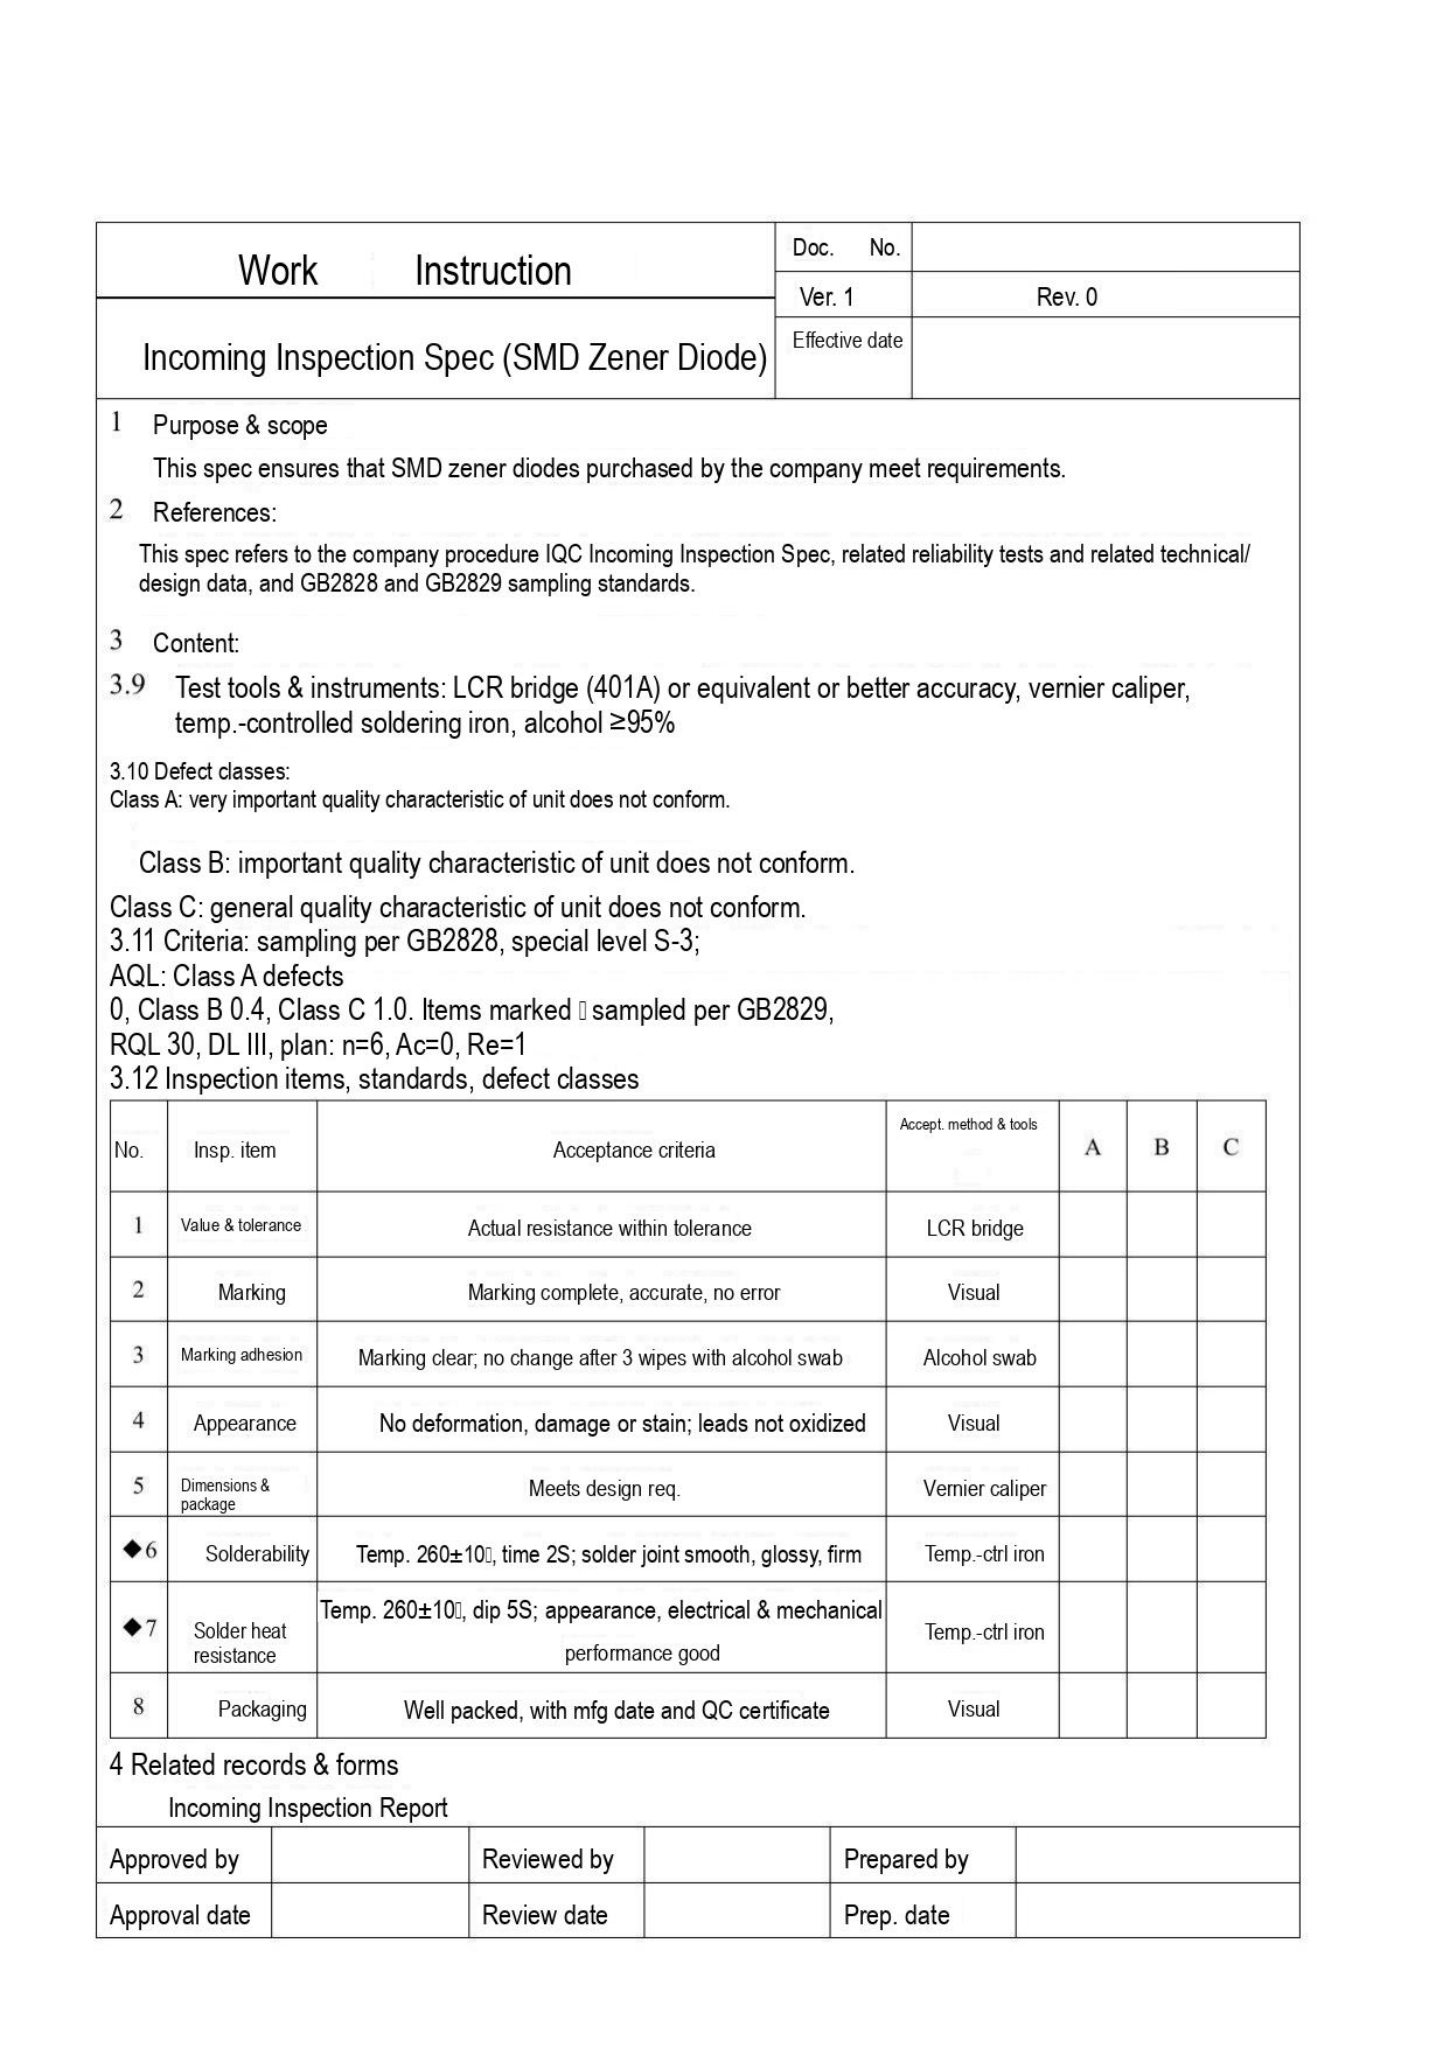# Work Instruction

| Doc. No. | |
|---|---|
| Ver. 1 | Rev. 0 |
| Effective date | |

Incoming Inspection Spec (SMD Zener Diode)

1 Purpose & scope

This spec ensures that SMD zener diodes purchased by the company meet requirements.

2 References:

This spec refers to the company procedure IQC Incoming Inspection Spec, related reliability tests and related technical/ design data, and GB2828 and GB2829 sampling standards.

3 Content:

3.9 Test tools & instruments: LCR bridge (401A) or equivalent or better accuracy, vernier caliper, temp.-controlled soldering iron, alcohol ≥95%

3.10 Defect classes:
Class A: very important quality characteristic of unit does not conform.

Class B: important quality characteristic of unit does not conform.

Class C: general quality characteristic of unit does not conform.
3.11 Criteria: sampling per GB2828, special level S-3;
AQL: Class A defects
0, Class B 0.4, Class C 1.0. Items marked sampled per GB2829,
RQL 30, DL III, plan: n=6, Ac=0, Re=1
3.12 Inspection items, standards, defect classes

| No. | Insp. item | Acceptance criteria | Accept. method & tools | A | B | C |
|---|---|---|---|---|---|---|
| 1 | Value & tolerance | Actual resistance within tolerance | LCR bridge | | | |
| 2 | Marking | Marking complete, accurate, no error | Visual | | | |
| 3 | Marking adhesion | Marking clear; no change after 3 wipes with alcohol swab | Alcohol swab | | | |
| 4 | Appearance | No deformation, damage or stain; leads not oxidized | Visual | | | |
| 5 | Dimensions & package | Meets design req. | Vernier caliper | | | |
| ◆6 | Solderability | Temp. 260±10, time 2S; solder joint smooth, glossy, firm | Temp.-ctrl iron | | | |
| ◆7 | Solder heat resistance | Temp. 260±10, dip 5S; appearance, electrical & mechanical performance good | Temp.-ctrl iron | | | |
| 8 | Packaging | Well packed, with mfg date and QC certificate | Visual | | | |

4 Related records & forms

Incoming Inspection Report

| Approved by | | Reviewed by | | Prepared by | |
|---|---|---|---|---|---|
| Approval date | | Review date | | Prep. date | |
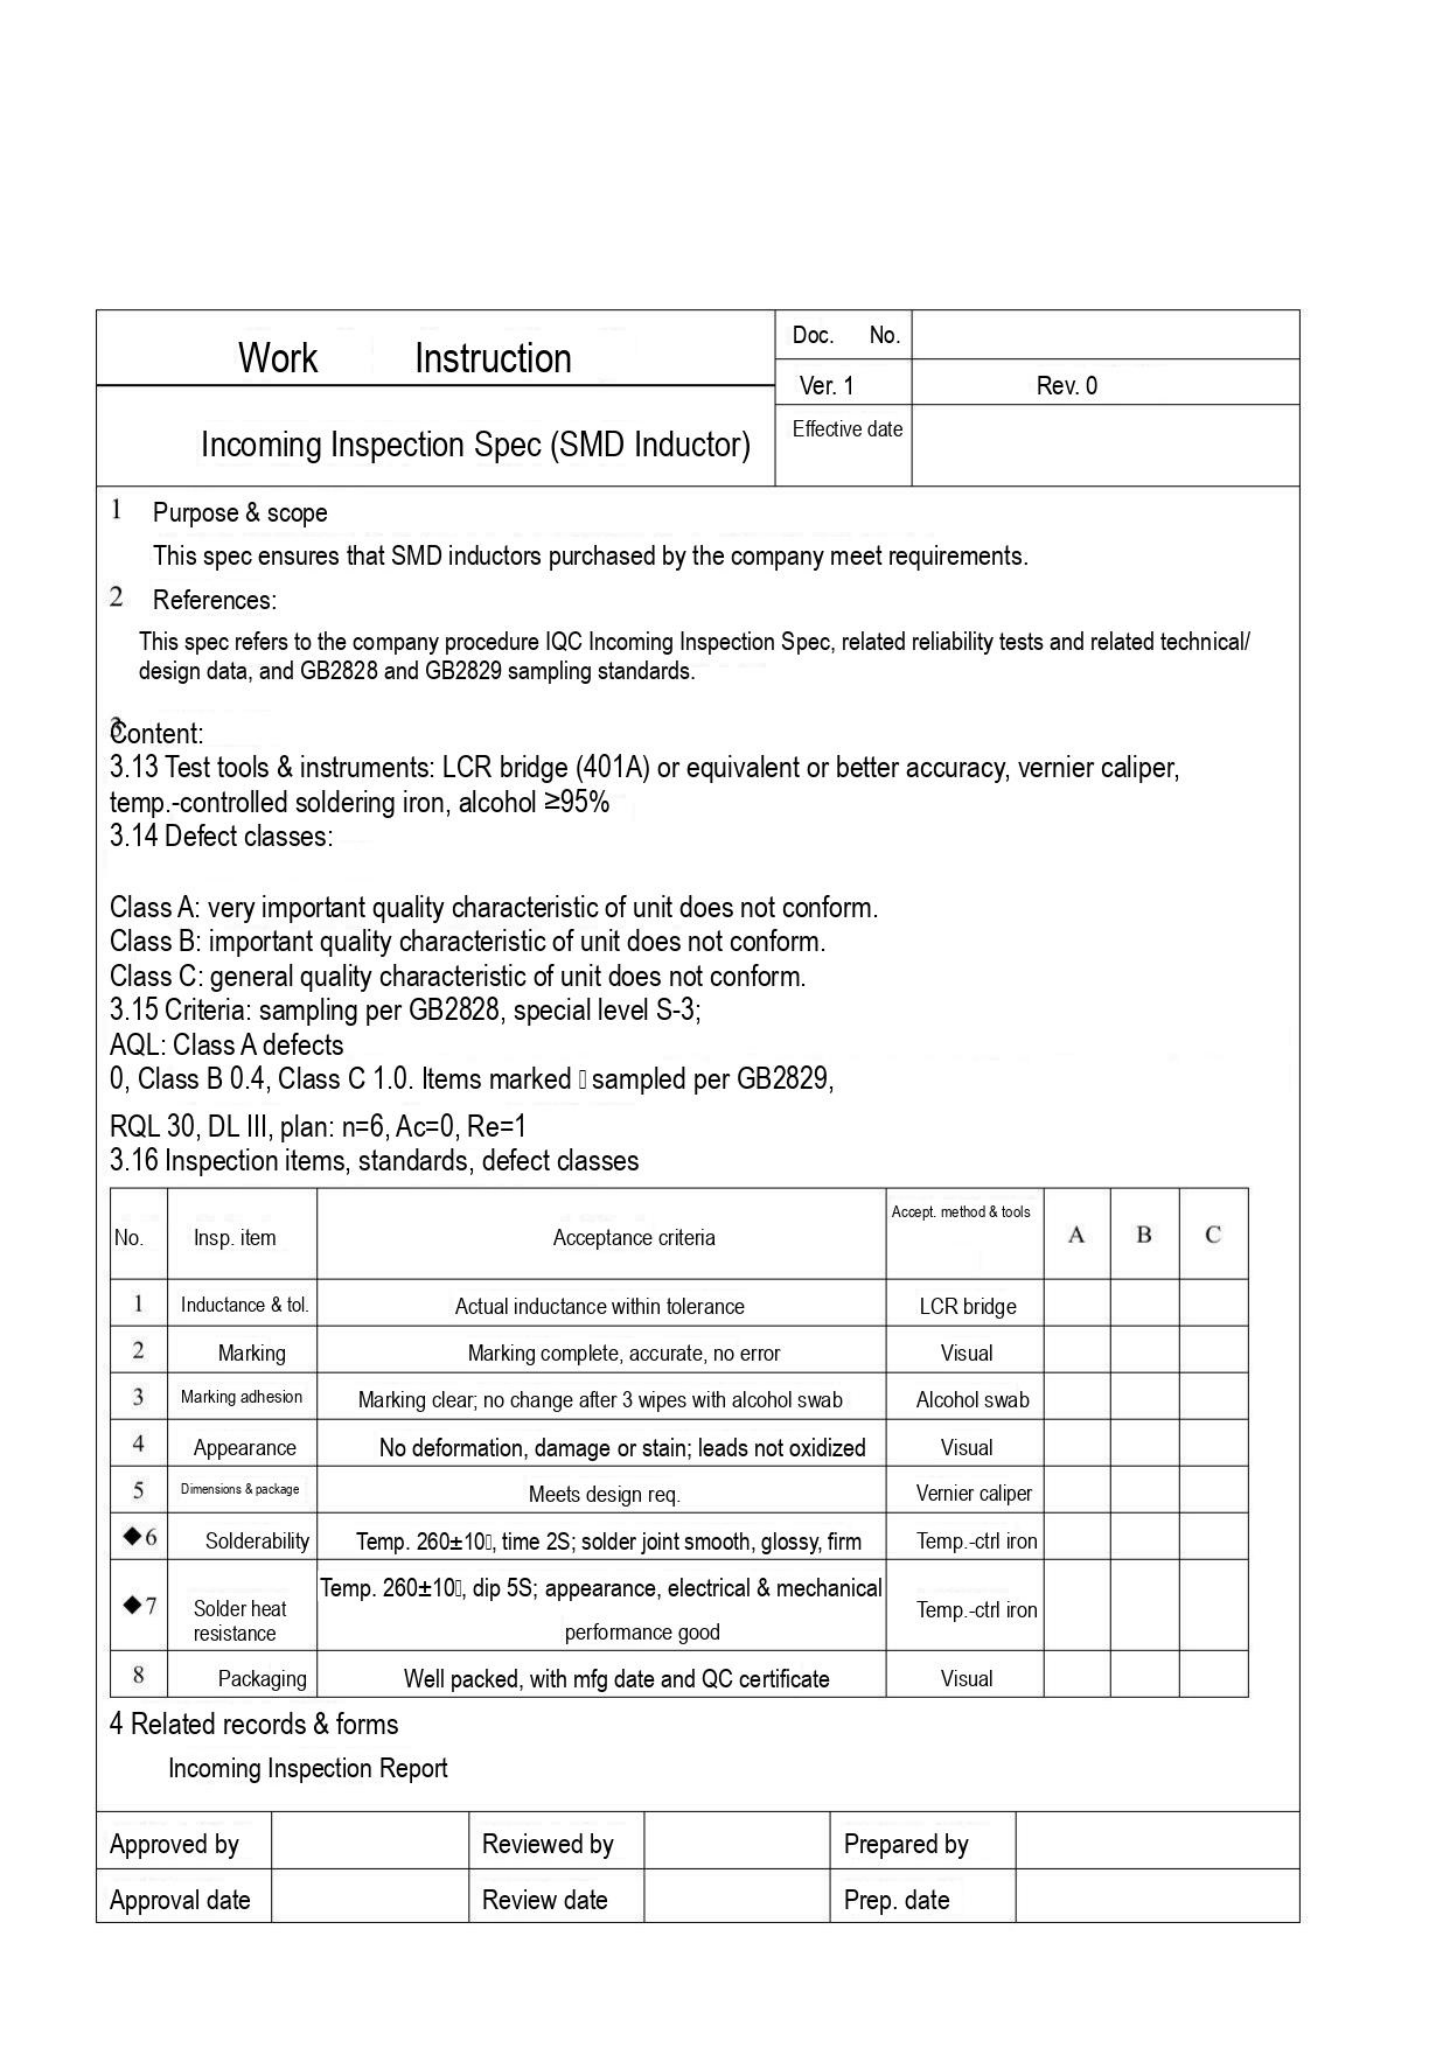| Work Instruction | Doc. No. | |
|---|---|---|
| | Ver. 1 | Rev. 0 |
| Incoming Inspection Spec (SMD Inductor) | Effective date | |

1 Purpose & scope

This spec ensures that SMD inductors purchased by the company meet requirements.

2 References:

This spec refers to the company procedure IQC Incoming Inspection Spec, related reliability tests and related technical/ design data, and GB2828 and GB2829 sampling standards.

3 Content:

3.13 Test tools & instruments: LCR bridge (401A) or equivalent or better accuracy, vernier caliper, temp.-controlled soldering iron, alcohol ≥95%

3.14 Defect classes:

Class A: very important quality characteristic of unit does not conform.
Class B: important quality characteristic of unit does not conform.
Class C: general quality characteristic of unit does not conform.

3.15 Criteria: sampling per GB2828, special level S-3;
AQL: Class A defects
0, Class B 0.4, Class C 1.0. Items marked sampled per GB2829,

RQL 30, DL III, plan: n=6, Ac=0, Re=1

3.16 Inspection items, standards, defect classes

| No. | Insp. item | Acceptance criteria | Accept. method & tools | A | B | C |
|---|---|---|---|---|---|---|
| 1 | Inductance & tol. | Actual inductance within tolerance | LCR bridge | | | |
| 2 | Marking | Marking complete, accurate, no error | Visual | | | |
| 3 | Marking adhesion | Marking clear; no change after 3 wipes with alcohol swab | Alcohol swab | | | |
| 4 | Appearance | No deformation, damage or stain; leads not oxidized | Visual | | | |
| 5 | Dimensions & package | Meets design req. | Vernier caliper | | | |
| ◆6 | Solderability | Temp. 260±10, time 2S; solder joint smooth, glossy, firm | Temp.-ctrl iron | | | |
| ◆7 | Solder heat resistance | Temp. 260±10, dip 5S; appearance, electrical & mechanical performance good | Temp.-ctrl iron | | | |
| 8 | Packaging | Well packed, with mfg date and QC certificate | Visual | | | |

4 Related records & forms

Incoming Inspection Report

| Approved by | | Reviewed by | | Prepared by | |
|---|---|---|---|---|---|
| Approval date | | Review date | | Prep. date | |
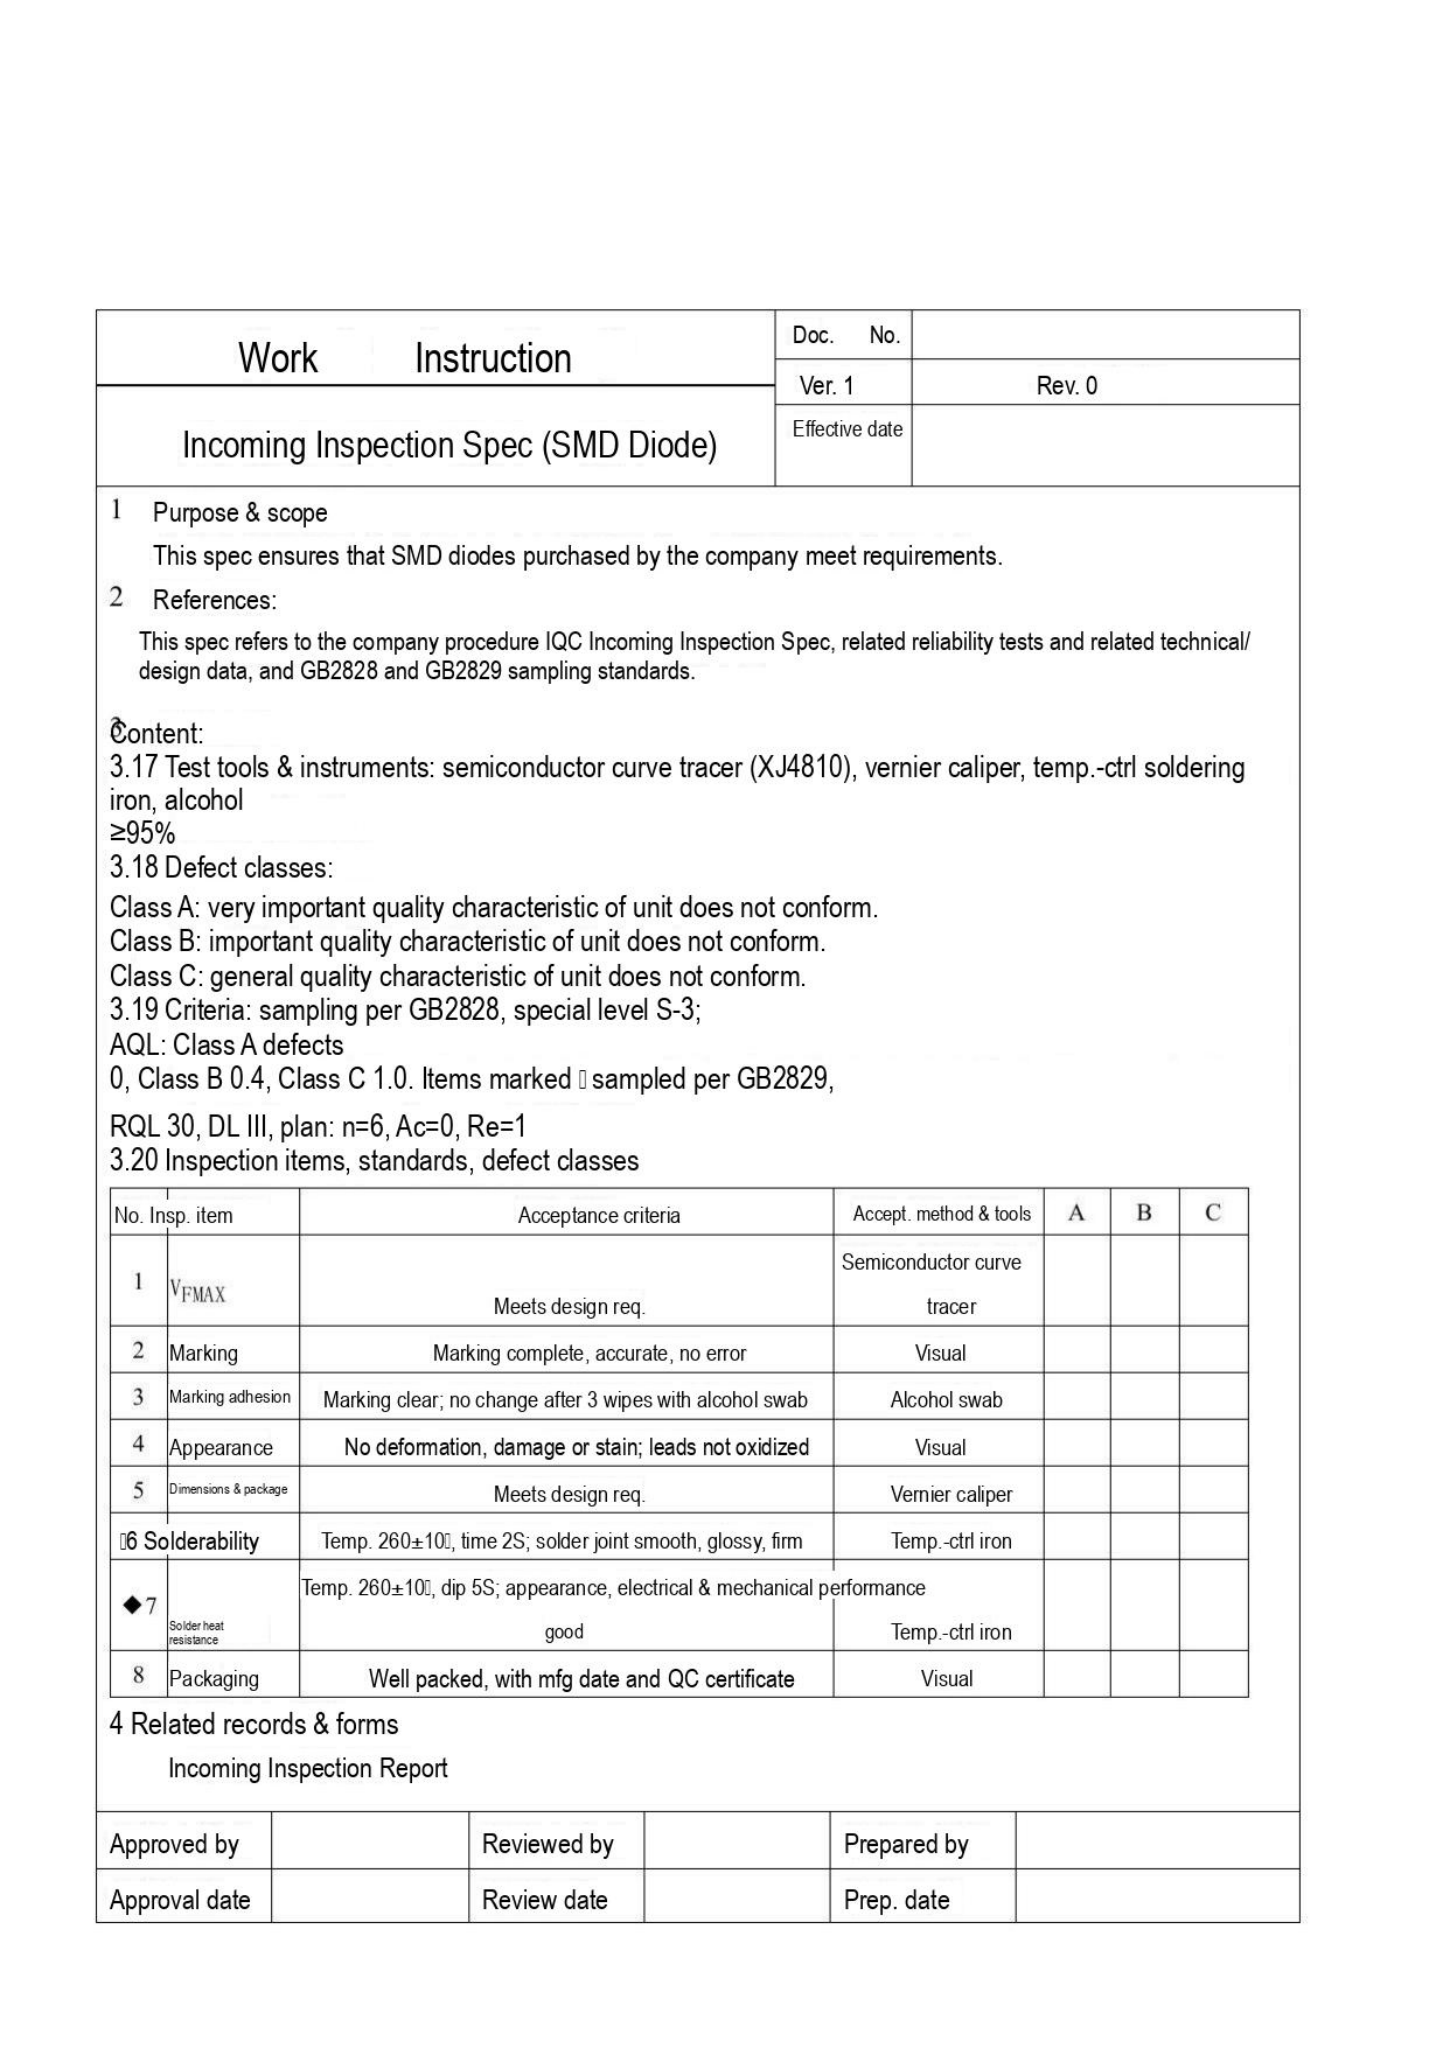| Work Instruction | Doc. No. | |
|---|---|---|
| | Ver. 1 | Rev. 0 |
| Incoming Inspection Spec (SMD Diode) | Effective date | |

1 Purpose & scope

This spec ensures that SMD diodes purchased by the company meet requirements.

2 References:

This spec refers to the company procedure IQC Incoming Inspection Spec, related reliability tests and related technical/design data, and GB2828 and GB2829 sampling standards.

3 Content:

3.17 Test tools & instruments: semiconductor curve tracer (XJ4810), vernier caliper, temp.-ctrl soldering iron, alcohol

≥95%

3.18 Defect classes:

Class A: very important quality characteristic of unit does not conform.

Class B: important quality characteristic of unit does not conform.

Class C: general quality characteristic of unit does not conform.

3.19 Criteria: sampling per GB2828, special level S-3;

AQL: Class A defects

0, Class B 0.4, Class C 1.0. Items marked sampled per GB2829,

RQL 30, DL III, plan: n=6, Ac=0, Re=1

3.20 Inspection items, standards, defect classes

| No. | Insp. item | Acceptance criteria | Accept. method & tools | A | B | C |
|---|---|---|---|---|---|---|
| 1 | V<sub>FMAX</sub> | Meets design req. | Semiconductor curve tracer | | | |
| 2 | Marking | Marking complete, accurate, no error | Visual | | | |
| 3 | Marking adhesion | Marking clear; no change after 3 wipes with alcohol swab | Alcohol swab | | | |
| 4 | Appearance | No deformation, damage or stain; leads not oxidized | Visual | | | |
| 5 | Dimensions & package | Meets design req. | Vernier caliper | | | |
| 6 | Solderability | Temp. 260±10, time 2S; solder joint smooth, glossy, firm | Temp.-ctrl iron | | | |
| ◆7 | Solder heat resistance | Temp. 260±10, dip 5S; appearance, electrical & mechanical performance good | Temp.-ctrl iron | | | |
| 8 | Packaging | Well packed, with mfg date and QC certificate | Visual | | | |

4 Related records & forms

Incoming Inspection Report

| Approved by | | Reviewed by | | Prepared by | |
|---|---|---|---|---|---|
| Approval date | | Review date | | Prep. date | |
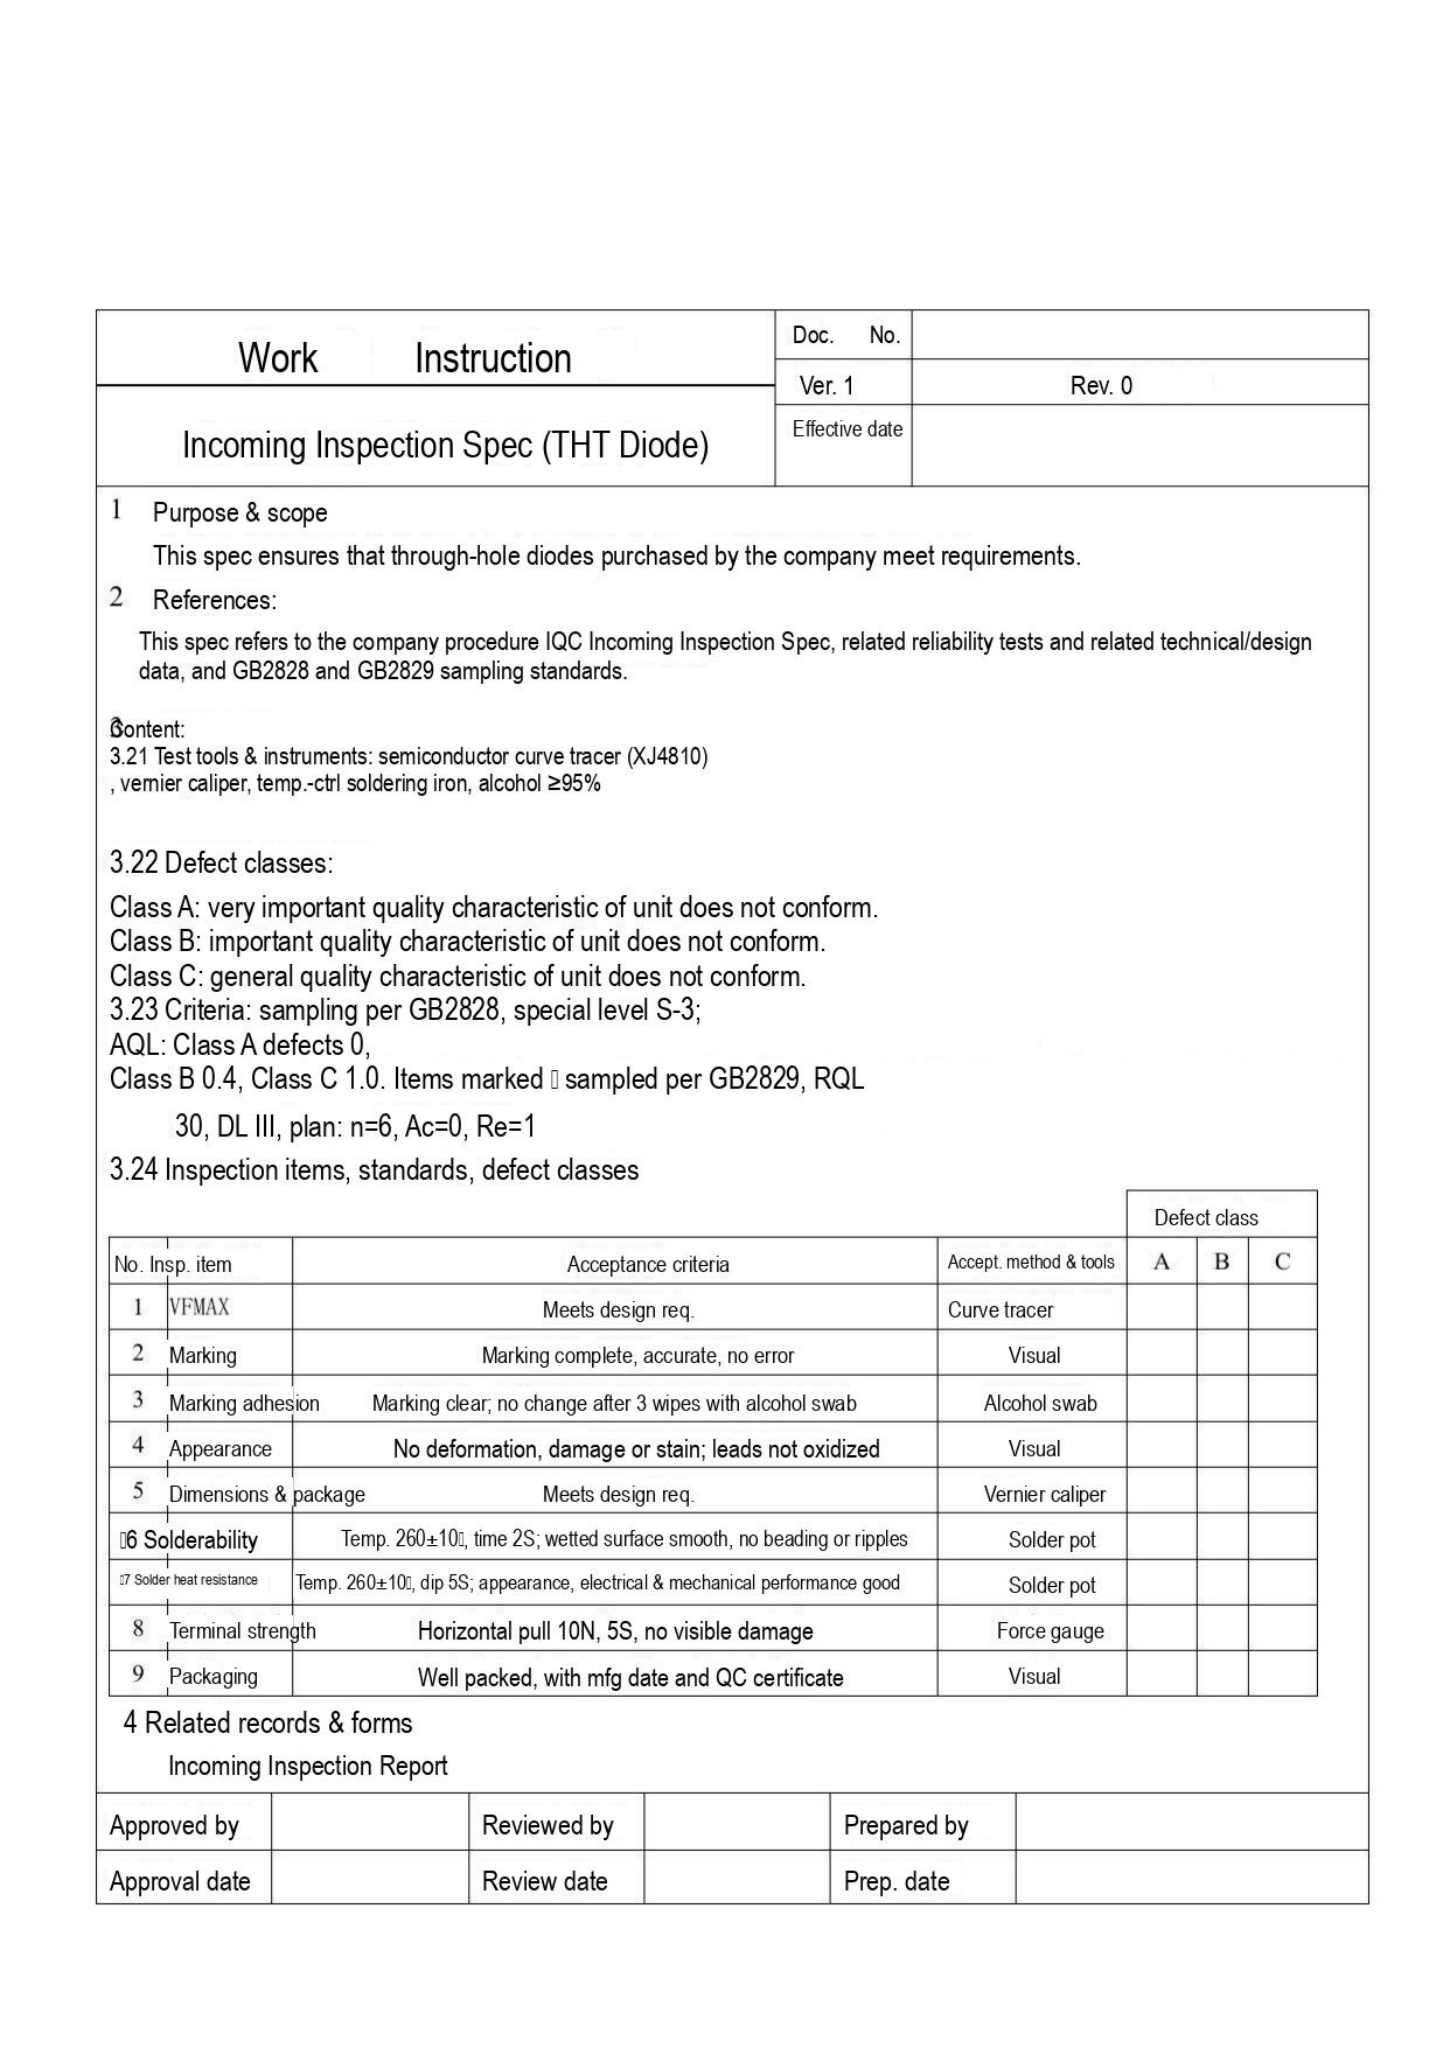| Work Instruction | Doc. No. | |
|---|---|---|
| | Ver. 1 | Rev. 0 |
| Incoming Inspection Spec (THT Diode) | Effective date | |

1 Purpose & scope

This spec ensures that through-hole diodes purchased by the company meet requirements.

2 References:

This spec refers to the company procedure IQC Incoming Inspection Spec, related reliability tests and related technical/design data, and GB2828 and GB2829 sampling standards.

3 Content:
3.21 Test tools & instruments: semiconductor curve tracer (XJ4810)
, vernier caliper, temp.-ctrl soldering iron, alcohol ≥95%

3.22 Defect classes:

Class A: very important quality characteristic of unit does not conform.
Class B: important quality characteristic of unit does not conform.
Class C: general quality characteristic of unit does not conform.
3.23 Criteria: sampling per GB2828, special level S-3;
AQL: Class A defects 0,
Class B 0.4, Class C 1.0. Items marked sampled per GB2829, RQL
30, DL III, plan: n=6, Ac=0, Re=1
3.24 Inspection items, standards, defect classes

| No. | Insp. item | Acceptance criteria | Accept. method & tools | Defect class A | Defect class B | Defect class C |
|---|---|---|---|---|---|---|
| 1 | VFMAX | Meets design req. | Curve tracer | | | |
| 2 | Marking | Marking complete, accurate, no error | Visual | | | |
| 3 | Marking adhesion | Marking clear; no change after 3 wipes with alcohol swab | Alcohol swab | | | |
| 4 | Appearance | No deformation, damage or stain; leads not oxidized | Visual | | | |
| 5 | Dimensions & package | Meets design req. | Vernier caliper | | | |
| 6 | Solderability | Temp. 260±10, time 2S; wetted surface smooth, no beading or ripples | Solder pot | | | |
| 7 | Solder heat resistance | Temp. 260±10, dip 5S; appearance, electrical & mechanical performance good | Solder pot | | | |
| 8 | Terminal strength | Horizontal pull 10N, 5S, no visible damage | Force gauge | | | |
| 9 | Packaging | Well packed, with mfg date and QC certificate | Visual | | | |

4 Related records & forms

Incoming Inspection Report

| Approved by | | Reviewed by | | Prepared by | |
|---|---|---|---|---|---|
| Approval date | | Review date | | Prep. date | |
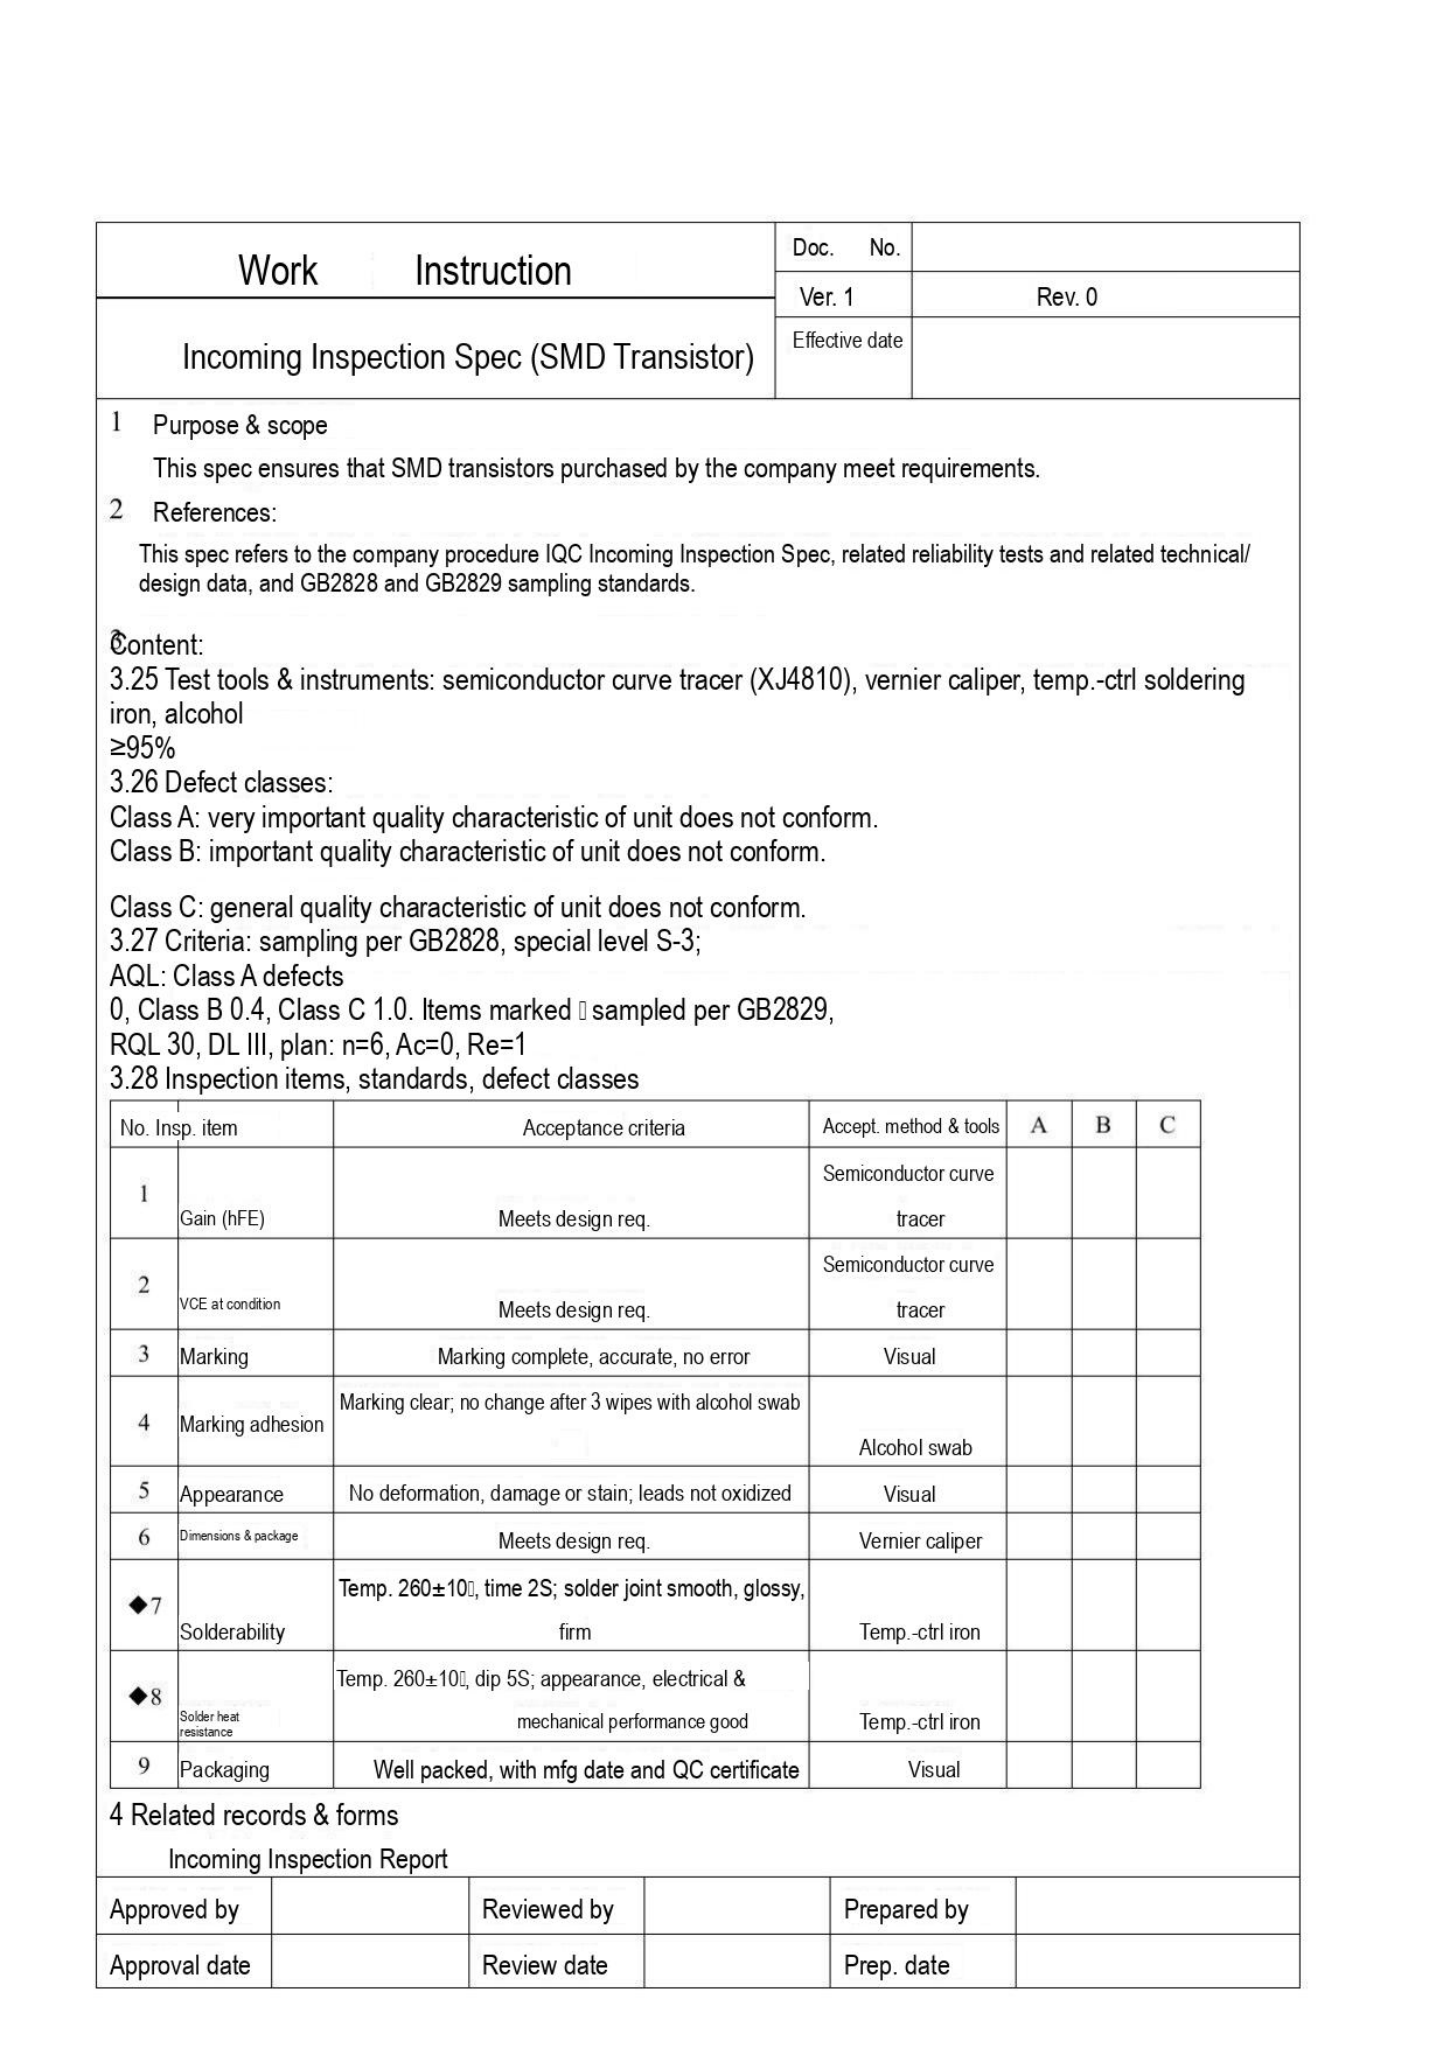| Work Instruction | Doc. No. | |
|---|---|---|
| | Ver. 1 | Rev. 0 |
| Incoming Inspection Spec (SMD Transistor) | Effective date | |

1 Purpose & scope

This spec ensures that SMD transistors purchased by the company meet requirements.

2 References:

This spec refers to the company procedure IQC Incoming Inspection Spec, related reliability tests and related technical/ design data, and GB2828 and GB2829 sampling standards.

3 Content:

3.25 Test tools & instruments: semiconductor curve tracer (XJ4810), vernier caliper, temp.-ctrl soldering iron, alcohol

≥95%

3.26 Defect classes:

Class A: very important quality characteristic of unit does not conform.

Class B: important quality characteristic of unit does not conform.

Class C: general quality characteristic of unit does not conform.

3.27 Criteria: sampling per GB2828, special level S-3;

AQL: Class A defects

0, Class B 0.4, Class C 1.0. Items marked sampled per GB2829,

RQL 30, DL III, plan: n=6, Ac=0, Re=1

3.28 Inspection items, standards, defect classes

| No. | Insp. item | Acceptance criteria | Accept. method & tools | A | B | C |
|---|---|---|---|---|---|---|
| 1 | Gain (hFE) | Meets design req. | Semiconductor curve tracer | | | |
| 2 | VCE at condition | Meets design req. | Semiconductor curve tracer | | | |
| 3 | Marking | Marking complete, accurate, no error | Visual | | | |
| 4 | Marking adhesion | Marking clear; no change after 3 wipes with alcohol swab | Alcohol swab | | | |
| 5 | Appearance | No deformation, damage or stain; leads not oxidized | Visual | | | |
| 6 | Dimensions & package | Meets design req. | Vernier caliper | | | |
| ◆7 | Solderability | Temp. 260±10, time 2S; solder joint smooth, glossy, firm | Temp.-ctrl iron | | | |
| ◆8 | Solder heat resistance | Temp. 260±10, dip 5S; appearance, electrical & mechanical performance good | Temp.-ctrl iron | | | |
| 9 | Packaging | Well packed, with mfg date and QC certificate | Visual | | | |

4 Related records & forms

Incoming Inspection Report

| Approved by | | Reviewed by | | Prepared by | |
|---|---|---|---|---|---|
| Approval date | | Review date | | Prep. date | |
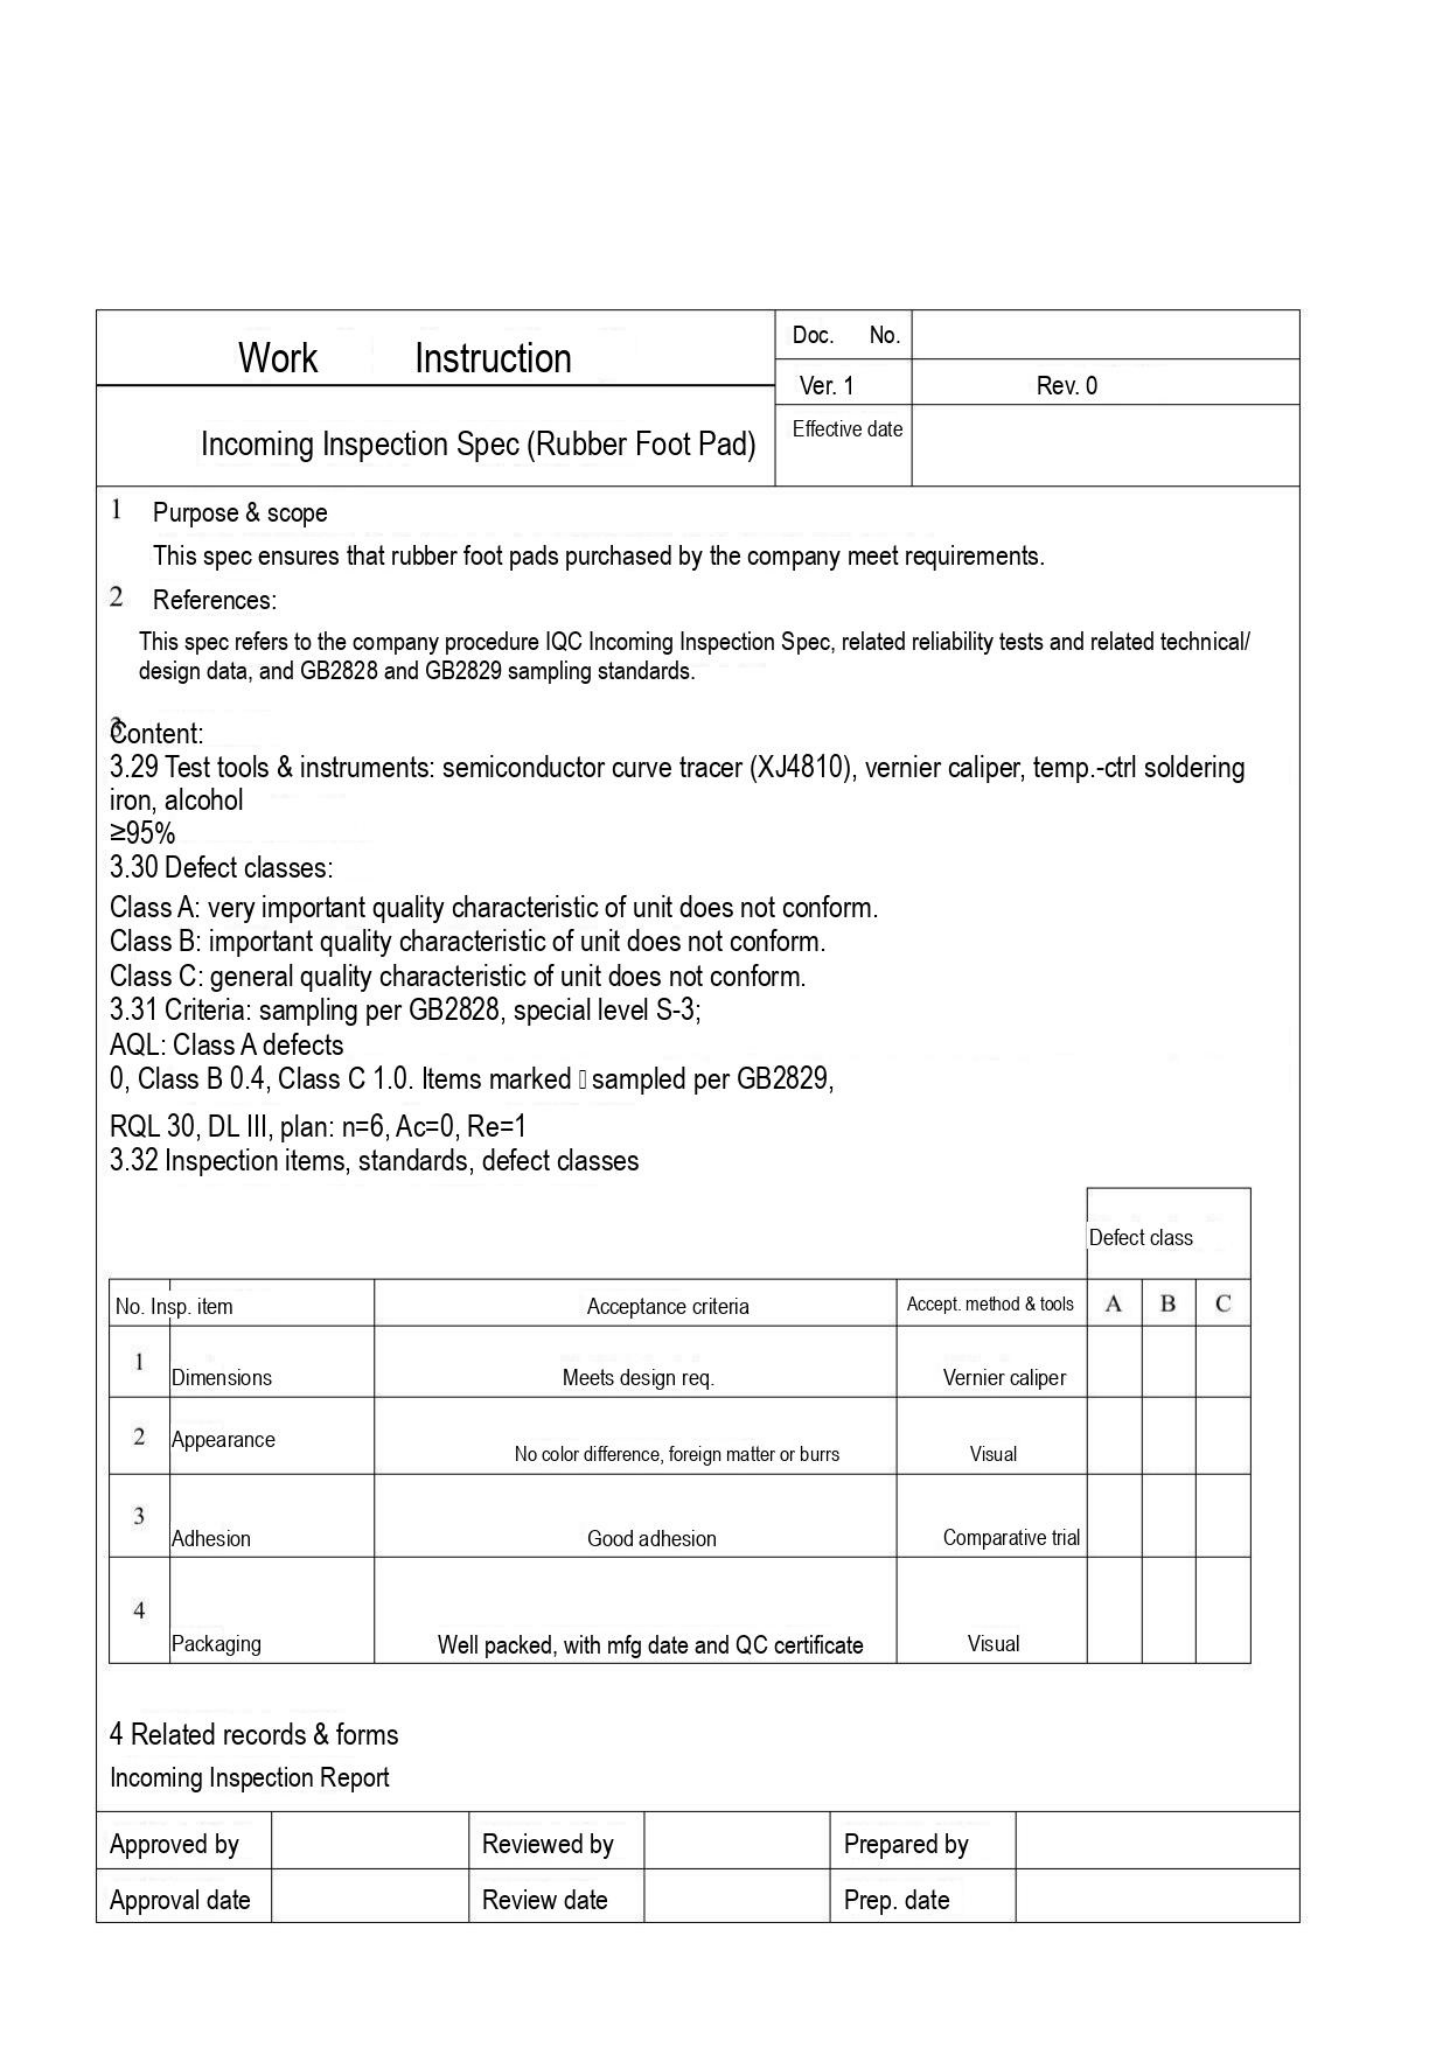| Work Instruction | Doc. No. | |
|---|---|---|
| | Ver. 1 | Rev. 0 |
| Incoming Inspection Spec (Rubber Foot Pad) | Effective date | |

1 Purpose & scope

This spec ensures that rubber foot pads purchased by the company meet requirements.

2 References:

This spec refers to the company procedure IQC Incoming Inspection Spec, related reliability tests and related technical/ design data, and GB2828 and GB2829 sampling standards.

3 Content:

3.29 Test tools & instruments: semiconductor curve tracer (XJ4810), vernier caliper, temp.-ctrl soldering iron, alcohol

≥95%

3.30 Defect classes:

Class A: very important quality characteristic of unit does not conform.

Class B: important quality characteristic of unit does not conform.

Class C: general quality characteristic of unit does not conform.

3.31 Criteria: sampling per GB2828, special level S-3;

AQL: Class A defects

0, Class B 0.4, Class C 1.0. Items marked sampled per GB2829,

RQL 30, DL III, plan: n=6, Ac=0, Re=1

3.32 Inspection items, standards, defect classes

| No. | Insp. item | Acceptance criteria | Accept. method & tools | Defect class A | Defect class B | Defect class C |
|---|---|---|---|---|---|---|
| 1 | Dimensions | Meets design req. | Vernier caliper | | | |
| 2 | Appearance | No color difference, foreign matter or burrs | Visual | | | |
| 3 | Adhesion | Good adhesion | Comparative trial | | | |
| 4 | Packaging | Well packed, with mfg date and QC certificate | Visual | | | |

4 Related records & forms

Incoming Inspection Report

| Approved by | | Reviewed by | | Prepared by | |
|---|---|---|---|---|---|
| Approval date | | Review date | | Prep. date | |